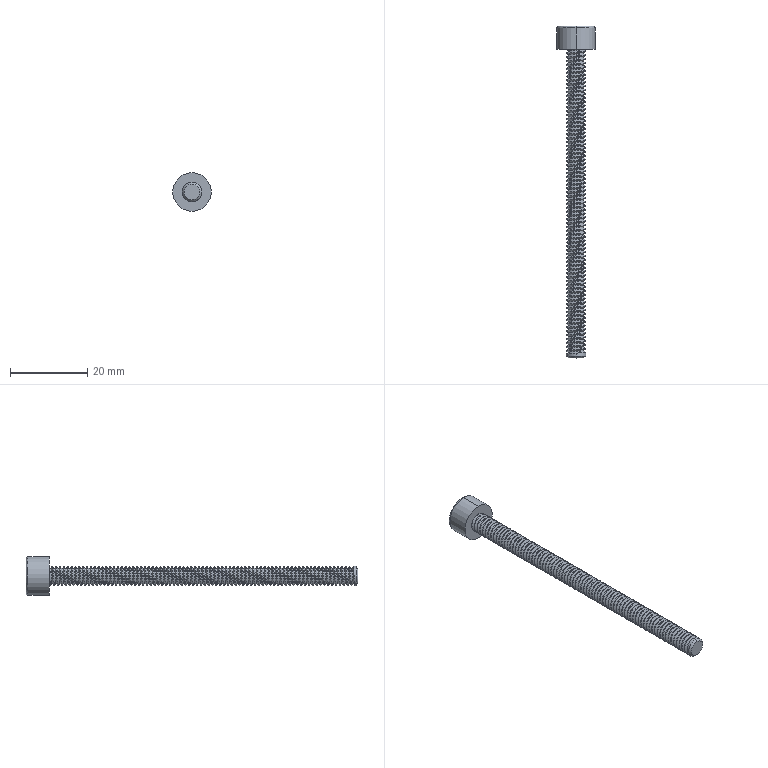Part | SolidWorks | features ICE 2, Chamfer 1, Extrusion 1, Fillet 1, SweepThread 1 | 1 solid | 185 faces | box 10 x 86 x 10 mm | volume 1649 mm3 | cylinder 166 | plane 12 | spline 3 | cone 2 | torus 2 | commonest cylinder face diameters 5.1 x164 10 x2